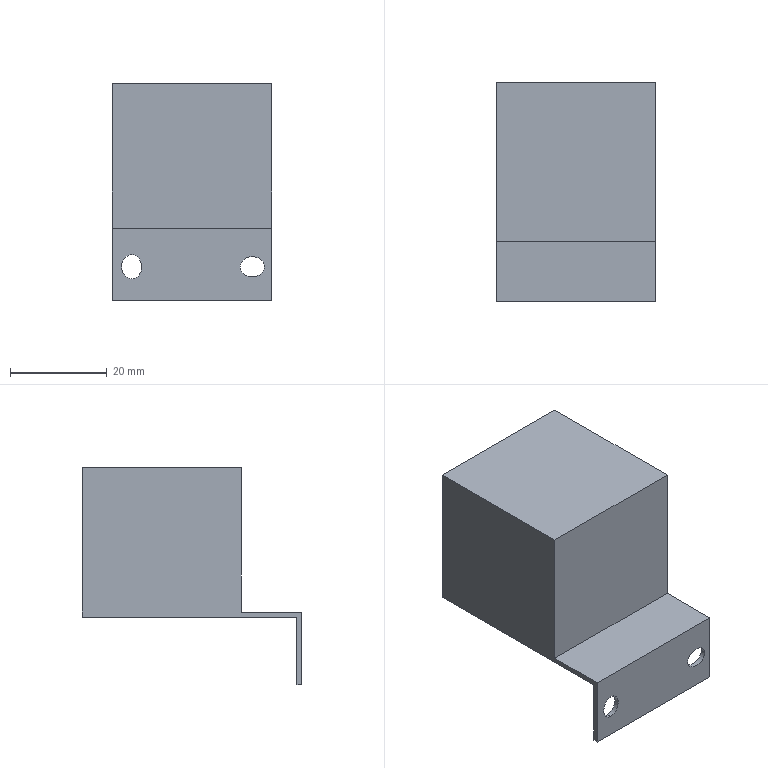Part | SolidWorks | features RefAxis 2, Boss 1, Cut 1, Extrusion 1 | 1 solid | 14 faces | box 33 x 45.5 x 45 mm | volume 34601 mm3 | plane 10 | spline 4
STEP:
#1=CARTESIAN_POINT('',(15.,-29.,-8.));
#2=VERTEX_POINT('',#1);
#3=CARTESIAN_POINT('',(10.,-29.,-8.));
#4=VERTEX_POINT('',#3);
#5=CARTESIAN_POINT('',(15.,-29.,-8.));
#6=CARTESIAN_POINT('',(15.,-29.,-12.2));
#7=CARTESIAN_POINT('',(10.,-29.,-12.2));
#8=CARTESIAN_POINT('',(10.,-29.,-8.));
#9=(BOUNDED_CURVE()B_SPLINE_CURVE(3,(#5,#6,#7,#8),.UNSPECIFIED.,.F.,.F.)B_SPLINE_CURVE_WITH_KNOTS((4,4),(3.142,6.283),.UNSPECIFIED.)CURVE()GEOMETRIC_REPRESENTATION_ITEM()RATIONAL_B_SPLINE_CURVE((1.,0.3333,0.3333,1.))REPRESENTATION_ITEM(''));
#10=EDGE_CURVE('',#2,#4,#9,.T.);
#11=ORIENTED_EDGE('',*,*,#10,.F.);
#12=CARTESIAN_POINT('',(15.,-28.,-8.));
#13=VERTEX_POINT('',#12);
#14=CARTESIAN_POINT('',(15.,-29.,-8.));
#15=DIRECTION('',(0.,1.,0.));
#16=VECTOR('',#15,1000.);
#17=LINE('',#14,#16);
#18=EDGE_CURVE('',#2,#13,#17,.T.);
#19=ORIENTED_EDGE('',*,*,#18,.T.);
#20=CARTESIAN_POINT('',(10.,-28.,-8.));
#21=VERTEX_POINT('',#20);
#22=CARTESIAN_POINT('',(15.,-28.,-8.));
#23=CARTESIAN_POINT('',(15.,-28.,-12.2));
#24=CARTESIAN_POINT('',(10.,-28.,-12.2));
#25=CARTESIAN_POINT('',(10.,-28.,-8.));
#26=(BOUNDED_CURVE()B_SPLINE_CURVE(3,(#22,#23,#24,#25),.UNSPECIFIED.,.F.,.F.)B_SPLINE_CURVE_WITH_KNOTS((4,4),(3.142,6.283),.UNSPECIFIED.)CURVE()GEOMETRIC_REPRESENTATION_ITEM()RATIONAL_B_SPLINE_CURVE((1.,0.3333,0.3333,1.))REPRESENTATION_ITEM(''));
#27=EDGE_CURVE('',#13,#21,#26,.T.);
#28=ORIENTED_EDGE('',*,*,#27,.T.);
#29=CARTESIAN_POINT('',(10.,-29.,-8.));
#30=DIRECTION('',(0.,1.,0.));
#31=VECTOR('',#30,1000.);
#32=LINE('',#29,#31);
#33=EDGE_CURVE('',#4,#21,#32,.T.);
#34=ORIENTED_EDGE('',*,*,#33,.F.);
#35=EDGE_LOOP('',(#11,#19,#28,#34));
#36=FACE_OUTER_BOUND('',#35,.T.);
#37=CARTESIAN_POINT('',(15.,-29.,-8.));
#38=CARTESIAN_POINT('',(15.,-28.,-8.));
#39=CARTESIAN_POINT('',(15.,-29.,-12.2));
#40=CARTESIAN_POINT('',(15.,-28.,-12.2));
#41=CARTESIAN_POINT('',(10.,-29.,-12.2));
#42=CARTESIAN_POINT('',(10.,-28.,-12.2));
#43=CARTESIAN_POINT('',(10.,-29.,-8.));
#44=CARTESIAN_POINT('',(10.,-28.,-8.));
#45=(BOUNDED_SURFACE()B_SPLINE_SURFACE(3,1,((#37,#38),(#39,#40),(#41,#42),(#43,#44)),.UNSPECIFIED.,.F.,.F.,.F.)B_SPLINE_SURFACE_WITH_KNOTS((4,4),(2,2),(0.,1.),(0.,1.),.UNSPECIFIED.)GEOMETRIC_REPRESENTATION_ITEM()RATIONAL_B_SPLINE_SURFACE(((1.,1.),(0.3333,0.3333),(0.3333,0.3333),(1.,1.)))REPRESENTATION_ITEM('')SURFACE());
#46=ADVANCED_FACE('',(#36),#45,.F.);
#47=CARTESIAN_POINT('',(-12.5,-29.,-5.5));
#48=VERTEX_POINT('',#47);
#49=CARTESIAN_POINT('',(-12.5,-29.,-10.5));
#50=VERTEX_POINT('',#49);
#51=CARTESIAN_POINT('',(-12.5,-29.,-5.5));
#52=CARTESIAN_POINT('',(-8.3,-29.,-5.5));
#53=CARTESIAN_POINT('',(-8.3,-29.,-10.5));
#54=CARTESIAN_POINT('',(-12.5,-29.,-10.5));
#55=(BOUNDED_CURVE()B_SPLINE_CURVE(3,(#51,#52,#53,#54),.UNSPECIFIED.,.F.,.F.)B_SPLINE_CURVE_WITH_KNOTS((4,4),(3.142,6.283),.UNSPECIFIED.)CURVE()GEOMETRIC_REPRESENTATION_ITEM()RATIONAL_B_SPLINE_CURVE((1.,0.3333,0.3333,1.))REPRESENTATION_ITEM(''));
#56=EDGE_CURVE('',#48,#50,#55,.T.);
#57=ORIENTED_EDGE('',*,*,#56,.F.);
#58=CARTESIAN_POINT('',(-12.5,-28.,-5.5));
#59=VERTEX_POINT('',#58);
#60=CARTESIAN_POINT('',(-12.5,-29.,-5.5));
#61=DIRECTION('',(0.,1.,0.));
#62=VECTOR('',#61,1000.);
#63=LINE('',#60,#62);
#64=EDGE_CURVE('',#48,#59,#63,.T.);
#65=ORIENTED_EDGE('',*,*,#64,.T.);
#66=CARTESIAN_POINT('',(-12.5,-28.,-10.5));
#67=VERTEX_POINT('',#66);
#68=CARTESIAN_POINT('',(-12.5,-28.,-5.5));
#69=CARTESIAN_POINT('',(-8.3,-28.,-5.5));
#70=CARTESIAN_POINT('',(-8.3,-28.,-10.5));
#71=CARTESIAN_POINT('',(-12.5,-28.,-10.5));
#72=(BOUNDED_CURVE()B_SPLINE_CURVE(3,(#68,#69,#70,#71),.UNSPECIFIED.,.F.,.F.)B_SPLINE_CURVE_WITH_KNOTS((4,4),(3.142,6.283),.UNSPECIFIED.)CURVE()GEOMETRIC_REPRESENTATION_ITEM()RATIONAL_B_SPLINE_CURVE((1.,0.3333,0.3333,1.))REPRESENTATION_ITEM(''));
#73=EDGE_CURVE('',#59,#67,#72,.T.);
#74=ORIENTED_EDGE('',*,*,#73,.T.);
#75=CARTESIAN_POINT('',(-12.5,-29.,-10.5));
#76=DIRECTION('',(0.,1.,0.));
#77=VECTOR('',#76,1000.);
#78=LINE('',#75,#77);
#79=EDGE_CURVE('',#50,#67,#78,.T.);
#80=ORIENTED_EDGE('',*,*,#79,.F.);
#81=EDGE_LOOP('',(#57,#65,#74,#80));
#82=FACE_OUTER_BOUND('',#81,.T.);
#83=CARTESIAN_POINT('',(-12.5,-29.,-5.5));
#84=CARTESIAN_POINT('',(-12.5,-28.,-5.5));
#85=CARTESIAN_POINT('',(-8.3,-29.,-5.5));
#86=CARTESIAN_POINT('',(-8.3,-28.,-5.5));
#87=CARTESIAN_POINT('',(-8.3,-29.,-10.5));
#88=CARTESIAN_POINT('',(-8.3,-28.,-10.5));
#89=CARTESIAN_POINT('',(-12.5,-29.,-10.5));
#90=CARTESIAN_POINT('',(-12.5,-28.,-10.5));
#91=(BOUNDED_SURFACE()B_SPLINE_SURFACE(3,1,((#83,#84),(#85,#86),(#87,#88),(#89,#90)),.UNSPECIFIED.,.F.,.F.,.T.)B_SPLINE_SURFACE_WITH_KNOTS((4,4),(2,2),(0.,1.),(0.,1.),.UNSPECIFIED.)GEOMETRIC_REPRESENTATION_ITEM()RATIONAL_B_SPLINE_SURFACE(((1.,1.),(0.3333,0.3333),(0.3333,0.3333),(1.,1.)))REPRESENTATION_ITEM('')SURFACE());
#92=ADVANCED_FACE('',(#82),#91,.F.);
#93=CARTESIAN_POINT('',(-16.5,16.5,30.));
#94=VERTEX_POINT('',#93);
#95=CARTESIAN_POINT('',(-16.5,16.5,-1.));
#96=VERTEX_POINT('',#95);
#97=CARTESIAN_POINT('',(-16.5,16.5,30.));
#98=DIRECTION('',(0.,0.,-1.));
#99=VECTOR('',#98,1000.);
#100=LINE('',#97,#99);
#101=EDGE_CURVE('',#94,#96,#100,.T.);
#102=ORIENTED_EDGE('',*,*,#101,.T.);
#103=CARTESIAN_POINT('',(-16.5,-28.,-1.));
#104=VERTEX_POINT('',#103);
#105=CARTESIAN_POINT('',(-16.5,-28.,-1.));
#106=DIRECTION('',(0.,1.,0.));
#107=VECTOR('',#106,1000.);
#108=LINE('',#105,#107);
#109=EDGE_CURVE('',#104,#96,#108,.T.);
#110=ORIENTED_EDGE('',*,*,#109,.F.);
#111=CARTESIAN_POINT('',(-16.5,-28.,-15.));
#112=VERTEX_POINT('',#111);
#113=CARTESIAN_POINT('',(-16.5,-28.,-15.));
#114=DIRECTION('',(0.,0.,1.));
#115=VECTOR('',#114,1000.);
#116=LINE('',#113,#115);
#117=EDGE_CURVE('',#112,#104,#116,.T.);
#118=ORIENTED_EDGE('',*,*,#117,.F.);
#119=CARTESIAN_POINT('',(-16.5,-29.,-15.));
#120=VERTEX_POINT('',#119);
#121=CARTESIAN_POINT('',(-16.5,-29.,-15.));
#122=DIRECTION('',(0.,1.,0.));
#123=VECTOR('',#122,1000.);
#124=LINE('',#121,#123);
#125=EDGE_CURVE('',#120,#112,#124,.T.);
#126=ORIENTED_EDGE('',*,*,#125,.F.);
#127=CARTESIAN_POINT('',(-16.5,-29.,0.));
#128=VERTEX_POINT('',#127);
#129=CARTESIAN_POINT('',(-16.5,-29.,0.));
#130=DIRECTION('',(0.,0.,-1.));
#131=VECTOR('',#130,1000.);
#132=LINE('',#129,#131);
#133=EDGE_CURVE('',#128,#120,#132,.T.);
#134=ORIENTED_EDGE('',*,*,#133,.F.);
#135=CARTESIAN_POINT('',(-16.5,-16.5,0.));
#136=VERTEX_POINT('',#135);
#137=CARTESIAN_POINT('',(-16.5,16.5,0.));
#138=DIRECTION('',(0.,-1.,0.));
#139=VECTOR('',#138,1000.);
#140=LINE('',#137,#139);
#141=EDGE_CURVE('',#136,#128,#140,.T.);
#142=ORIENTED_EDGE('',*,*,#141,.F.);
#143=CARTESIAN_POINT('',(-16.5,-16.5,30.));
#144=VERTEX_POINT('',#143);
#145=CARTESIAN_POINT('',(-16.5,-16.5,30.));
#146=DIRECTION('',(0.,0.,-1.));
#147=VECTOR('',#146,1000.);
#148=LINE('',#145,#147);
#149=EDGE_CURVE('',#144,#136,#148,.T.);
#150=ORIENTED_EDGE('',*,*,#149,.F.);
#151=CARTESIAN_POINT('',(-16.5,16.5,30.));
#152=DIRECTION('',(0.,-1.,0.));
#153=VECTOR('',#152,1000.);
#154=LINE('',#151,#153);
#155=EDGE_CURVE('',#94,#144,#154,.T.);
#156=ORIENTED_EDGE('',*,*,#155,.F.);
#157=EDGE_LOOP('',(#102,#110,#118,#126,#134,#142,#150,#156));
#158=FACE_OUTER_BOUND('',#157,.T.);
#159=CARTESIAN_POINT('',(-16.5,16.5,30.));
#160=DIRECTION('',(1.,0.,0.));
#161=DIRECTION('',(0.,1.,0.));
#162=AXIS2_PLACEMENT_3D('',#159,#160,#161);
#163=PLANE('',#162);
#164=ADVANCED_FACE('',(#158),#163,.F.);
#165=CARTESIAN_POINT('',(16.5,-16.5,0.));
#166=VERTEX_POINT('',#165);
#167=CARTESIAN_POINT('',(-16.5,-16.5,0.));
#168=DIRECTION('',(1.,0.,0.));
#169=VECTOR('',#168,1000.);
#170=LINE('',#167,#169);
#171=EDGE_CURVE('',#136,#166,#170,.T.);
#172=ORIENTED_EDGE('',*,*,#171,.T.);
#173=CARTESIAN_POINT('',(16.5,-16.5,30.));
#174=VERTEX_POINT('',#173);
#175=CARTESIAN_POINT('',(16.5,-16.5,30.));
#176=DIRECTION('',(0.,0.,-1.));
#177=VECTOR('',#176,1000.);
#178=LINE('',#175,#177);
#179=EDGE_CURVE('',#174,#166,#178,.T.);
#180=ORIENTED_EDGE('',*,*,#179,.F.);
#181=CARTESIAN_POINT('',(-16.5,-16.5,30.));
#182=DIRECTION('',(1.,0.,0.));
#183=VECTOR('',#182,1000.);
#184=LINE('',#181,#183);
#185=EDGE_CURVE('',#144,#174,#184,.T.);
#186=ORIENTED_EDGE('',*,*,#185,.F.);
#187=ORIENTED_EDGE('',*,*,#149,.T.);
#188=EDGE_LOOP('',(#172,#180,#186,#187));
#189=FACE_OUTER_BOUND('',#188,.T.);
#190=CARTESIAN_POINT('',(-16.5,-16.5,30.));
#191=DIRECTION('',(0.,1.,0.));
#192=DIRECTION('',(-1.,0.,0.));
#193=AXIS2_PLACEMENT_3D('',#190,#191,#192);
#194=PLANE('',#193);
#195=ADVANCED_FACE('',(#189),#194,.F.);
#196=ORIENTED_EDGE('',*,*,#179,.T.);
#197=CARTESIAN_POINT('',(16.5,-29.,0.));
#198=VERTEX_POINT('',#197);
#199=CARTESIAN_POINT('',(16.5,16.5,0.));
#200=DIRECTION('',(0.,-1.,0.));
#201=VECTOR('',#200,1000.);
#202=LINE('',#199,#201);
#203=EDGE_CURVE('',#166,#198,#202,.T.);
#204=ORIENTED_EDGE('',*,*,#203,.T.);
#205=CARTESIAN_POINT('',(16.5,-29.,-15.));
#206=VERTEX_POINT('',#205);
#207=CARTESIAN_POINT('',(16.5,-29.,0.));
#208=DIRECTION('',(0.,0.,-1.));
#209=VECTOR('',#208,1000.);
#210=LINE('',#207,#209);
#211=EDGE_CURVE('',#198,#206,#210,.T.);
#212=ORIENTED_EDGE('',*,*,#211,.T.);
#213=CARTESIAN_POINT('',(16.5,-28.,-15.));
#214=VERTEX_POINT('',#213);
#215=CARTESIAN_POINT('',(16.5,-29.,-15.));
#216=DIRECTION('',(0.,1.,0.));
#217=VECTOR('',#216,1000.);
#218=LINE('',#215,#217);
#219=EDGE_CURVE('',#206,#214,#218,.T.);
#220=ORIENTED_EDGE('',*,*,#219,.T.);
#221=CARTESIAN_POINT('',(16.5,-28.,-1.));
#222=VERTEX_POINT('',#221);
#223=CARTESIAN_POINT('',(16.5,-28.,-15.));
#224=DIRECTION('',(0.,0.,1.));
#225=VECTOR('',#224,1000.);
#226=LINE('',#223,#225);
#227=EDGE_CURVE('',#214,#222,#226,.T.);
#228=ORIENTED_EDGE('',*,*,#227,.T.);
#229=CARTESIAN_POINT('',(16.5,16.5,-1.));
#230=VERTEX_POINT('',#229);
#231=CARTESIAN_POINT('',(16.5,-28.,-1.));
#232=DIRECTION('',(0.,1.,0.));
#233=VECTOR('',#232,1000.);
#234=LINE('',#231,#233);
#235=EDGE_CURVE('',#222,#230,#234,.T.);
#236=ORIENTED_EDGE('',*,*,#235,.T.);
#237=CARTESIAN_POINT('',(16.5,16.5,30.));
#238=VERTEX_POINT('',#237);
#239=CARTESIAN_POINT('',(16.5,16.5,30.));
#240=DIRECTION('',(0.,0.,-1.));
#241=VECTOR('',#240,1000.);
#242=LINE('',#239,#241);
#243=EDGE_CURVE('',#238,#230,#242,.T.);
#244=ORIENTED_EDGE('',*,*,#243,.F.);
#245=CARTESIAN_POINT('',(16.5,16.5,30.));
#246=DIRECTION('',(0.,1.,0.));
#247=VECTOR('',#246,1000.);
#248=LINE('',#245,#247);
#249=EDGE_CURVE('',#174,#238,#248,.T.);
#250=ORIENTED_EDGE('',*,*,#249,.F.);
#251=EDGE_LOOP('',(#196,#204,#212,#220,#228,#236,#244,#250));
#252=FACE_OUTER_BOUND('',#251,.T.);
#253=CARTESIAN_POINT('',(16.5,16.5,30.));
#254=DIRECTION('',(-1.,0.,0.));
#255=DIRECTION('',(0.,-1.,0.));
#256=AXIS2_PLACEMENT_3D('',#253,#254,#255);
#257=PLANE('',#256);
#258=ADVANCED_FACE('',(#252),#257,.F.);
#259=ORIENTED_EDGE('',*,*,#243,.T.);
#260=CARTESIAN_POINT('',(16.5,16.5,-1.));
#261=DIRECTION('',(-1.,0.,0.));
#262=VECTOR('',#261,1000.);
#263=LINE('',#260,#262);
#264=EDGE_CURVE('',#230,#96,#263,.T.);
#265=ORIENTED_EDGE('',*,*,#264,.T.);
#266=ORIENTED_EDGE('',*,*,#101,.F.);
#267=CARTESIAN_POINT('',(-16.5,16.5,30.));
#268=DIRECTION('',(-1.,0.,0.));
#269=VECTOR('',#268,1000.);
#270=LINE('',#267,#269);
#271=EDGE_CURVE('',#238,#94,#270,.T.);
#272=ORIENTED_EDGE('',*,*,#271,.F.);
#273=EDGE_LOOP('',(#259,#265,#266,#272));
#274=FACE_OUTER_BOUND('',#273,.T.);
#275=CARTESIAN_POINT('',(-16.5,16.5,30.));
#276=DIRECTION('',(0.,-1.,0.));
#277=DIRECTION('',(0.,0.,-1.));
#278=AXIS2_PLACEMENT_3D('',#275,#276,#277);
#279=PLANE('',#278);
#280=ADVANCED_FACE('',(#274),#279,.F.);
#281=ORIENTED_EDGE('',*,*,#155,.T.);
#282=ORIENTED_EDGE('',*,*,#185,.T.);
#283=ORIENTED_EDGE('',*,*,#249,.T.);
#284=ORIENTED_EDGE('',*,*,#271,.T.);
#285=EDGE_LOOP('',(#281,#282,#283,#284));
#286=FACE_OUTER_BOUND('',#285,.T.);
#287=CARTESIAN_POINT('',(-16.5,-16.5,30.));
#288=DIRECTION('',(0.,0.,1.));
#289=DIRECTION('',(1.,0.,0.));
#290=AXIS2_PLACEMENT_3D('',#287,#288,#289);
#291=PLANE('',#290);
#292=ADVANCED_FACE('',(#286),#291,.T.);
#293=ORIENTED_EDGE('',*,*,#171,.F.);
#294=ORIENTED_EDGE('',*,*,#141,.T.);
#295=CARTESIAN_POINT('',(16.5,-29.,0.));
#296=DIRECTION('',(-1.,0.,0.));
#297=VECTOR('',#296,1000.);
#298=LINE('',#295,#297);
#299=EDGE_CURVE('',#198,#128,#298,.T.);
#300=ORIENTED_EDGE('',*,*,#299,.F.);
#301=ORIENTED_EDGE('',*,*,#203,.F.);
#302=EDGE_LOOP('',(#293,#294,#300,#301));
#303=FACE_OUTER_BOUND('',#302,.T.);
#304=CARTESIAN_POINT('',(16.5,16.5,0.));
#305=DIRECTION('',(0.,0.,-1.));
#306=DIRECTION('',(0.,1.,0.));
#307=AXIS2_PLACEMENT_3D('',#304,#305,#306);
#308=PLANE('',#307);
#309=ADVANCED_FACE('',(#303),#308,.F.);
#310=CARTESIAN_POINT('',(10.,-29.,-8.));
#311=CARTESIAN_POINT('',(10.,-29.,-3.8));
#312=CARTESIAN_POINT('',(15.,-29.,-3.8));
#313=CARTESIAN_POINT('',(15.,-29.,-8.));
#314=(BOUNDED_CURVE()B_SPLINE_CURVE(3,(#310,#311,#312,#313),.UNSPECIFIED.,.F.,.F.)B_SPLINE_CURVE_WITH_KNOTS((4,4),(0.,3.142),.UNSPECIFIED.)CURVE()GEOMETRIC_REPRESENTATION_ITEM()RATIONAL_B_SPLINE_CURVE((1.,0.3333,0.3333,1.))REPRESENTATION_ITEM(''));
#315=EDGE_CURVE('',#4,#2,#314,.T.);
#316=ORIENTED_EDGE('',*,*,#315,.T.);
#317=ORIENTED_EDGE('',*,*,#10,.T.);
#318=EDGE_LOOP('',(#316,#317));
#319=FACE_BOUND('',#318,.T.);
#320=CARTESIAN_POINT('',(-12.5,-29.,-10.5));
#321=CARTESIAN_POINT('',(-16.7,-29.,-10.5));
#322=CARTESIAN_POINT('',(-16.7,-29.,-5.5));
#323=CARTESIAN_POINT('',(-12.5,-29.,-5.5));
#324=(BOUNDED_CURVE()B_SPLINE_CURVE(3,(#320,#321,#322,#323),.UNSPECIFIED.,.F.,.F.)B_SPLINE_CURVE_WITH_KNOTS((4,4),(0.,3.142),.UNSPECIFIED.)CURVE()GEOMETRIC_REPRESENTATION_ITEM()RATIONAL_B_SPLINE_CURVE((1.,0.3333,0.3333,1.))REPRESENTATION_ITEM(''));
#325=EDGE_CURVE('',#50,#48,#324,.T.);
#326=ORIENTED_EDGE('',*,*,#325,.T.);
#327=ORIENTED_EDGE('',*,*,#56,.T.);
#328=EDGE_LOOP('',(#326,#327));
#329=FACE_BOUND('',#328,.T.);
#330=ORIENTED_EDGE('',*,*,#133,.T.);
#331=CARTESIAN_POINT('',(16.5,-29.,-15.));
#332=DIRECTION('',(-1.,0.,0.));
#333=VECTOR('',#332,1000.);
#334=LINE('',#331,#333);
#335=EDGE_CURVE('',#206,#120,#334,.T.);
#336=ORIENTED_EDGE('',*,*,#335,.F.);
#337=ORIENTED_EDGE('',*,*,#211,.F.);
#338=ORIENTED_EDGE('',*,*,#299,.T.);
#339=EDGE_LOOP('',(#330,#336,#337,#338));
#340=FACE_OUTER_BOUND('',#339,.T.);
#341=CARTESIAN_POINT('',(16.5,-29.,0.));
#342=DIRECTION('',(0.,1.,0.));
#343=DIRECTION('',(0.,0.,1.));
#344=AXIS2_PLACEMENT_3D('',#341,#342,#343);
#345=PLANE('',#344);
#346=ADVANCED_FACE('',(#319,#329,#340),#345,.F.);
#347=ORIENTED_EDGE('',*,*,#125,.T.);
#348=CARTESIAN_POINT('',(16.5,-28.,-15.));
#349=DIRECTION('',(-1.,0.,0.));
#350=VECTOR('',#349,1000.);
#351=LINE('',#348,#350);
#352=EDGE_CURVE('',#214,#112,#351,.T.);
#353=ORIENTED_EDGE('',*,*,#352,.F.);
#354=ORIENTED_EDGE('',*,*,#219,.F.);
#355=ORIENTED_EDGE('',*,*,#335,.T.);
#356=EDGE_LOOP('',(#347,#353,#354,#355));
#357=FACE_OUTER_BOUND('',#356,.T.);
#358=CARTESIAN_POINT('',(16.5,-29.,-15.));
#359=DIRECTION('',(0.,0.,1.));
#360=DIRECTION('',(1.,0.,0.));
#361=AXIS2_PLACEMENT_3D('',#358,#359,#360);
#362=PLANE('',#361);
#363=ADVANCED_FACE('',(#357),#362,.F.);
#364=CARTESIAN_POINT('',(10.,-28.,-8.));
#365=CARTESIAN_POINT('',(10.,-28.,-3.8));
#366=CARTESIAN_POINT('',(15.,-28.,-3.8));
#367=CARTESIAN_POINT('',(15.,-28.,-8.));
#368=(BOUNDED_CURVE()B_SPLINE_CURVE(3,(#364,#365,#366,#367),.UNSPECIFIED.,.F.,.F.)B_SPLINE_CURVE_WITH_KNOTS((4,4),(0.,3.142),.UNSPECIFIED.)CURVE()GEOMETRIC_REPRESENTATION_ITEM()RATIONAL_B_SPLINE_CURVE((1.,0.3333,0.3333,1.))REPRESENTATION_ITEM(''));
#369=EDGE_CURVE('',#21,#13,#368,.T.);
#370=ORIENTED_EDGE('',*,*,#369,.F.);
#371=ORIENTED_EDGE('',*,*,#27,.F.);
#372=EDGE_LOOP('',(#370,#371));
#373=FACE_BOUND('',#372,.T.);
#374=CARTESIAN_POINT('',(-12.5,-28.,-10.5));
#375=CARTESIAN_POINT('',(-16.7,-28.,-10.5));
#376=CARTESIAN_POINT('',(-16.7,-28.,-5.5));
#377=CARTESIAN_POINT('',(-12.5,-28.,-5.5));
#378=(BOUNDED_CURVE()B_SPLINE_CURVE(3,(#374,#375,#376,#377),.UNSPECIFIED.,.F.,.T.)B_SPLINE_CURVE_WITH_KNOTS((4,4),(0.,3.142),.UNSPECIFIED.)CURVE()GEOMETRIC_REPRESENTATION_ITEM()RATIONAL_B_SPLINE_CURVE((1.,0.3333,0.3333,1.))REPRESENTATION_ITEM(''));
#379=EDGE_CURVE('',#67,#59,#378,.T.);
#380=ORIENTED_EDGE('',*,*,#379,.F.);
#381=ORIENTED_EDGE('',*,*,#73,.F.);
#382=EDGE_LOOP('',(#380,#381));
#383=FACE_BOUND('',#382,.T.);
#384=ORIENTED_EDGE('',*,*,#117,.T.);
#385=CARTESIAN_POINT('',(16.5,-28.,-1.));
#386=DIRECTION('',(-1.,0.,0.));
#387=VECTOR('',#386,1000.);
#388=LINE('',#385,#387);
#389=EDGE_CURVE('',#222,#104,#388,.T.);
#390=ORIENTED_EDGE('',*,*,#389,.F.);
#391=ORIENTED_EDGE('',*,*,#227,.F.);
#392=ORIENTED_EDGE('',*,*,#352,.T.);
#393=EDGE_LOOP('',(#384,#390,#391,#392));
#394=FACE_OUTER_BOUND('',#393,.T.);
#395=CARTESIAN_POINT('',(16.5,-28.,-15.));
#396=DIRECTION('',(0.,-1.,0.));
#397=DIRECTION('',(0.,0.,-1.));
#398=AXIS2_PLACEMENT_3D('',#395,#396,#397);
#399=PLANE('',#398);
#400=ADVANCED_FACE('',(#373,#383,#394),#399,.F.);
#401=ORIENTED_EDGE('',*,*,#109,.T.);
#402=ORIENTED_EDGE('',*,*,#264,.F.);
#403=ORIENTED_EDGE('',*,*,#235,.F.);
#404=ORIENTED_EDGE('',*,*,#389,.T.);
#405=EDGE_LOOP('',(#401,#402,#403,#404));
#406=FACE_OUTER_BOUND('',#405,.T.);
#407=CARTESIAN_POINT('',(16.5,-28.,-1.));
#408=DIRECTION('',(0.,0.,1.));
#409=DIRECTION('',(1.,0.,0.));
#410=AXIS2_PLACEMENT_3D('',#407,#408,#409);
#411=PLANE('',#410);
#412=ADVANCED_FACE('',(#406),#411,.F.);
#413=ORIENTED_EDGE('',*,*,#64,.F.);
#414=ORIENTED_EDGE('',*,*,#325,.F.);
#415=ORIENTED_EDGE('',*,*,#79,.T.);
#416=ORIENTED_EDGE('',*,*,#379,.T.);
#417=EDGE_LOOP('',(#413,#414,#415,#416));
#418=FACE_OUTER_BOUND('',#417,.T.);
#419=CARTESIAN_POINT('',(-12.5,-29.,-10.5));
#420=CARTESIAN_POINT('',(-12.5,-28.,-10.5));
#421=CARTESIAN_POINT('',(-16.7,-29.,-10.5));
#422=CARTESIAN_POINT('',(-16.7,-28.,-10.5));
#423=CARTESIAN_POINT('',(-16.7,-29.,-5.5));
#424=CARTESIAN_POINT('',(-16.7,-28.,-5.5));
#425=CARTESIAN_POINT('',(-12.5,-29.,-5.5));
#426=CARTESIAN_POINT('',(-12.5,-28.,-5.5));
#427=(BOUNDED_SURFACE()B_SPLINE_SURFACE(3,1,((#419,#420),(#421,#422),(#423,#424),(#425,#426)),.UNSPECIFIED.,.F.,.F.,.T.)B_SPLINE_SURFACE_WITH_KNOTS((4,4),(2,2),(0.,1.),(0.,1.),.UNSPECIFIED.)GEOMETRIC_REPRESENTATION_ITEM()RATIONAL_B_SPLINE_SURFACE(((1.,1.),(0.3333,0.3333),(0.3333,0.3333),(1.,1.)))REPRESENTATION_ITEM('')SURFACE());
#428=ADVANCED_FACE('',(#418),#427,.F.);
#429=ORIENTED_EDGE('',*,*,#18,.F.);
#430=ORIENTED_EDGE('',*,*,#315,.F.);
#431=ORIENTED_EDGE('',*,*,#33,.T.);
#432=ORIENTED_EDGE('',*,*,#369,.T.);
#433=EDGE_LOOP('',(#429,#430,#431,#432));
#434=FACE_OUTER_BOUND('',#433,.T.);
#435=CARTESIAN_POINT('',(10.,-29.,-8.));
#436=CARTESIAN_POINT('',(10.,-28.,-8.));
#437=CARTESIAN_POINT('',(10.,-29.,-3.8));
#438=CARTESIAN_POINT('',(10.,-28.,-3.8));
#439=CARTESIAN_POINT('',(15.,-29.,-3.8));
#440=CARTESIAN_POINT('',(15.,-28.,-3.8));
#441=CARTESIAN_POINT('',(15.,-29.,-8.));
#442=CARTESIAN_POINT('',(15.,-28.,-8.));
#443=(BOUNDED_SURFACE()B_SPLINE_SURFACE(3,1,((#435,#436),(#437,#438),(#439,#440),(#441,#442)),.UNSPECIFIED.,.F.,.F.,.T.)B_SPLINE_SURFACE_WITH_KNOTS((4,4),(2,2),(0.,1.),(0.,1.),.UNSPECIFIED.)GEOMETRIC_REPRESENTATION_ITEM()RATIONAL_B_SPLINE_SURFACE(((1.,1.),(0.3333,0.3333),(0.3333,0.3333),(1.,1.)))REPRESENTATION_ITEM('')SURFACE());
#444=ADVANCED_FACE('',(#434),#443,.F.);
#445=CLOSED_SHELL('',(#46,#92,#164,#195,#258,#280,#292,#309,#346,#363,#400,#412,#428,#444));
#446=MANIFOLD_SOLID_BREP('',#445);
#447=CARTESIAN_POINT('',(0.,0.,0.));
#448=DIRECTION('',(0.,0.,1.));
#449=DIRECTION('',(1.,0.,0.));
#450=AXIS2_PLACEMENT_3D('',#447,#448,#449);
#451=(LENGTH_UNIT()NAMED_UNIT(*)SI_UNIT(.MILLI.,.METRE.));
#452=UNCERTAINTY_MEASURE_WITH_UNIT(LENGTH_MEASURE(0.00001),#451,'','');
#453=(NAMED_UNIT(*)PLANE_ANGLE_UNIT()SI_UNIT($,.RADIAN.));
#454=(NAMED_UNIT(*)SI_UNIT($,.STERADIAN.)SOLID_ANGLE_UNIT());
#455=(GEOMETRIC_REPRESENTATION_CONTEXT(3)GLOBAL_UNCERTAINTY_ASSIGNED_CONTEXT((#452))GLOBAL_UNIT_ASSIGNED_CONTEXT((#451,#453,#454))REPRESENTATION_CONTEXT('',''));
#456=ADVANCED_BREP_SHAPE_REPRESENTATION('',(#446,#450),#455);